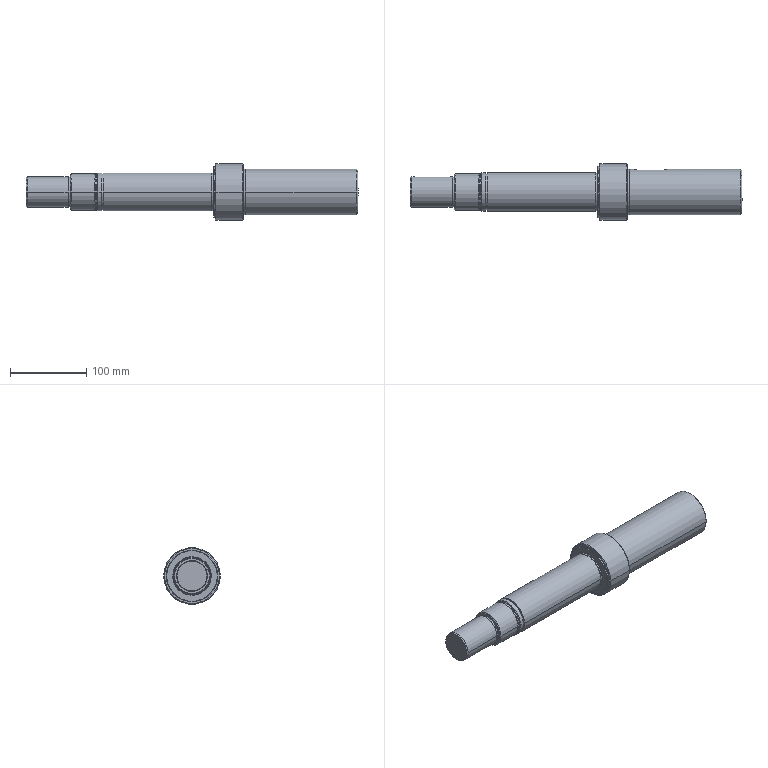Part | SolidWorks | features BaseBody 1 | 1 solid | 88 faces | box 434.34 x 74 x 74 mm | volume 1002154 mm3 | cylinder 31 | cone 26 | spline 16 | plane 15 | commonest cylinder face diameters 50 x4 40 x3 12 x2 17.294 x2 18 x2 39.5 x2